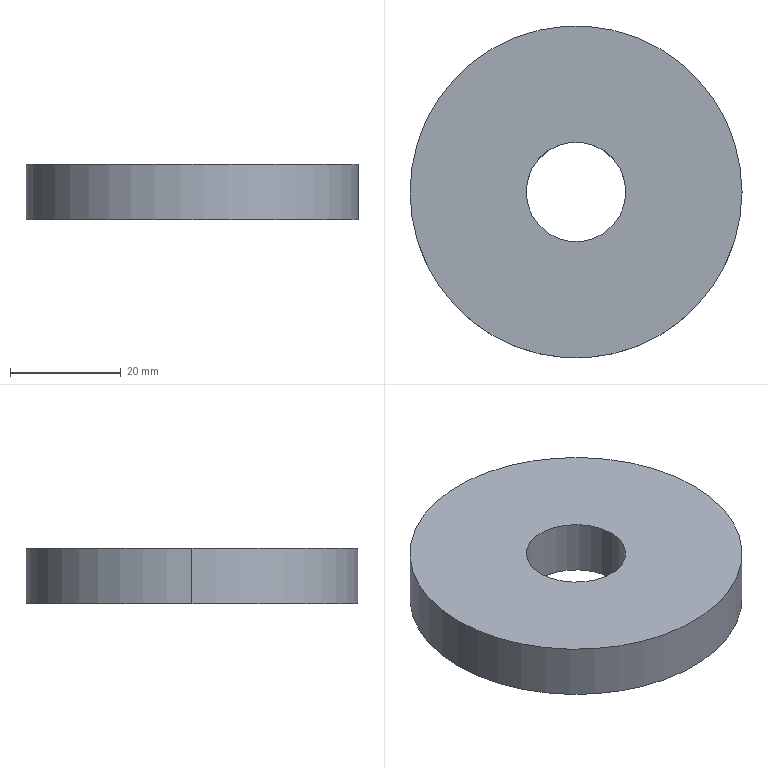Part | STEP file | Pressing pad | 1 solid | 6 faces | box 60 x 60 x 10 mm | volume 25730 mm3 | cylinder 4 | plane 2 | commonest cylinder face diameters 18 x2 60 x2
STEP:
#1=CARTESIAN_POINT('',(0.,0.,0.));
#2=DIRECTION('',(0.,0.,1.));
#3=DIRECTION('',(1.,0.,0.));
#4=AXIS2_PLACEMENT_3D('',#1,#2,#3);
#5=CARTESIAN_POINT('',(-9.,0.,10.));
#6=VERTEX_POINT('',#5);
#7=CARTESIAN_POINT('',(-9.,0.,0.));
#8=VERTEX_POINT('',#7);
#9=CARTESIAN_POINT('',(-9.,0.,10.));
#10=DIRECTION('',(0.,0.,-1.));
#11=VECTOR('',#10,1.);
#12=LINE('',#9,#11);
#13=CARTESIAN_POINT('',(0.,0.,10.));
#14=DIRECTION('',(0.,0.,-1.));
#15=DIRECTION('',(-1.,0.,0.));
#16=AXIS2_PLACEMENT_3D('',#13,#14,#15);
#17=CYLINDRICAL_SURFACE('',#16,9.);
#18=CARTESIAN_POINT('',(6.283,0.));
#19=DIRECTION('',(0.,1.));
#20=VECTOR('',#19,1.);
#21=LINE('',#18,#20);
#22=(GEOMETRIC_REPRESENTATION_CONTEXT(2)PARAMETRIC_REPRESENTATION_CONTEXT()REPRESENTATION_CONTEXT('',''));
#23=DEFINITIONAL_REPRESENTATION('',(#21),#22);
#24=PCURVE('',#17,#23);
#25=CARTESIAN_POINT('',(0.,0.,10.));
#26=DIRECTION('',(0.,0.,-1.));
#27=DIRECTION('',(-1.,0.,0.));
#28=AXIS2_PLACEMENT_3D('',#25,#26,#27);
#29=CYLINDRICAL_SURFACE('',#28,9.);
#30=CARTESIAN_POINT('',(0.,0.));
#31=DIRECTION('',(0.,1.));
#32=VECTOR('',#31,1.);
#33=LINE('',#30,#32);
#34=(GEOMETRIC_REPRESENTATION_CONTEXT(2)PARAMETRIC_REPRESENTATION_CONTEXT()REPRESENTATION_CONTEXT('',''));
#35=DEFINITIONAL_REPRESENTATION('',(#33),#34);
#36=PCURVE('',#29,#35);
#37=SURFACE_CURVE('',#12,(#24,#36),.PCURVE_S1.);
#38=EDGE_CURVE('',#6,#8,#37,.T.);
#39=ORIENTED_EDGE('',*,*,#38,.T.);
#40=CARTESIAN_POINT('',(9.,0.,0.));
#41=VERTEX_POINT('',#40);
#42=CARTESIAN_POINT('',(0.,0.,0.));
#43=DIRECTION('',(0.,0.,1.));
#44=DIRECTION('',(1.,0.,0.));
#45=AXIS2_PLACEMENT_3D('',#42,#43,#44);
#46=CIRCLE('',#45,9.);
#47=CARTESIAN_POINT('',(9.425,10.));
#48=DIRECTION('',(-1.,0.));
#49=VECTOR('',#48,1.);
#50=LINE('',#47,#49);
#51=(GEOMETRIC_REPRESENTATION_CONTEXT(2)PARAMETRIC_REPRESENTATION_CONTEXT()REPRESENTATION_CONTEXT('',''));
#52=DEFINITIONAL_REPRESENTATION('',(#50),#51);
#53=PCURVE('',#17,#52);
#54=CARTESIAN_POINT('',(0.,0.,0.));
#55=DIRECTION('',(0.,0.,1.));
#56=DIRECTION('',(1.,0.,0.));
#57=AXIS2_PLACEMENT_3D('',#54,#55,#56);
#58=PLANE('',#57);
#59=CARTESIAN_POINT('',(0.,0.));
#60=DIRECTION('',(1.,0.));
#61=AXIS2_PLACEMENT_2D('',#59,#60);
#62=CIRCLE('',#61,9.);
#63=(GEOMETRIC_REPRESENTATION_CONTEXT(2)PARAMETRIC_REPRESENTATION_CONTEXT()REPRESENTATION_CONTEXT('',''));
#64=DEFINITIONAL_REPRESENTATION('',(#62),#63);
#65=PCURVE('',#58,#64);
#66=SURFACE_CURVE('',#46,(#53,#65),.PCURVE_S1.);
#67=EDGE_CURVE('',#8,#41,#66,.T.);
#68=ORIENTED_EDGE('',*,*,#67,.T.);
#69=CARTESIAN_POINT('',(9.,0.,10.));
#70=VERTEX_POINT('',#69);
#71=CARTESIAN_POINT('',(9.,0.,10.));
#72=DIRECTION('',(0.,0.,-1.));
#73=VECTOR('',#72,1.);
#74=LINE('',#71,#73);
#75=CARTESIAN_POINT('',(3.142,0.));
#76=DIRECTION('',(0.,1.));
#77=VECTOR('',#76,1.);
#78=LINE('',#75,#77);
#79=(GEOMETRIC_REPRESENTATION_CONTEXT(2)PARAMETRIC_REPRESENTATION_CONTEXT()REPRESENTATION_CONTEXT('',''));
#80=DEFINITIONAL_REPRESENTATION('',(#78),#79);
#81=PCURVE('',#17,#80);
#82=CARTESIAN_POINT('',(3.142,0.));
#83=DIRECTION('',(0.,1.));
#84=VECTOR('',#83,1.);
#85=LINE('',#82,#84);
#86=(GEOMETRIC_REPRESENTATION_CONTEXT(2)PARAMETRIC_REPRESENTATION_CONTEXT()REPRESENTATION_CONTEXT('',''));
#87=DEFINITIONAL_REPRESENTATION('',(#85),#86);
#88=PCURVE('',#29,#87);
#89=SURFACE_CURVE('',#74,(#81,#88),.PCURVE_S1.);
#90=EDGE_CURVE('',#70,#41,#89,.T.);
#91=ORIENTED_EDGE('',*,*,#90,.F.);
#92=CARTESIAN_POINT('',(0.,0.,10.));
#93=DIRECTION('',(0.,0.,1.));
#94=DIRECTION('',(1.,0.,0.));
#95=AXIS2_PLACEMENT_3D('',#92,#93,#94);
#96=CIRCLE('',#95,9.);
#97=CARTESIAN_POINT('',(9.425,0.));
#98=DIRECTION('',(-1.,0.));
#99=VECTOR('',#98,1.);
#100=LINE('',#97,#99);
#101=(GEOMETRIC_REPRESENTATION_CONTEXT(2)PARAMETRIC_REPRESENTATION_CONTEXT()REPRESENTATION_CONTEXT('',''));
#102=DEFINITIONAL_REPRESENTATION('',(#100),#101);
#103=PCURVE('',#17,#102);
#104=CARTESIAN_POINT('',(0.,0.,10.));
#105=DIRECTION('',(0.,0.,1.));
#106=DIRECTION('',(1.,0.,0.));
#107=AXIS2_PLACEMENT_3D('',#104,#105,#106);
#108=PLANE('',#107);
#109=CARTESIAN_POINT('',(0.,0.));
#110=DIRECTION('',(1.,0.));
#111=AXIS2_PLACEMENT_2D('',#109,#110);
#112=CIRCLE('',#111,9.);
#113=(GEOMETRIC_REPRESENTATION_CONTEXT(2)PARAMETRIC_REPRESENTATION_CONTEXT()REPRESENTATION_CONTEXT('',''));
#114=DEFINITIONAL_REPRESENTATION('',(#112),#113);
#115=PCURVE('',#108,#114);
#116=SURFACE_CURVE('',#96,(#103,#115),.PCURVE_S1.);
#117=EDGE_CURVE('',#6,#70,#116,.T.);
#118=ORIENTED_EDGE('',*,*,#117,.F.);
#119=EDGE_LOOP('',(#39,#68,#91,#118));
#120=FACE_BOUND('',#119,.F.);
#121=ADVANCED_FACE('',(#120),#17,.F.);
#122=CARTESIAN_POINT('',(30.,0.,10.));
#123=VERTEX_POINT('',#122);
#124=CARTESIAN_POINT('',(-30.,0.,10.));
#125=VERTEX_POINT('',#124);
#126=CARTESIAN_POINT('',(0.,0.,10.));
#127=DIRECTION('',(0.,0.,1.));
#128=DIRECTION('',(1.,0.,0.));
#129=AXIS2_PLACEMENT_3D('',#126,#127,#128);
#130=CIRCLE('',#129,30.);
#131=CARTESIAN_POINT('',(0.,0.,10.));
#132=DIRECTION('',(0.,0.,-1.));
#133=DIRECTION('',(-1.,0.,0.));
#134=AXIS2_PLACEMENT_3D('',#131,#132,#133);
#135=CYLINDRICAL_SURFACE('',#134,30.);
#136=CARTESIAN_POINT('',(3.142,0.));
#137=DIRECTION('',(-1.,0.));
#138=VECTOR('',#137,1.);
#139=LINE('',#136,#138);
#140=(GEOMETRIC_REPRESENTATION_CONTEXT(2)PARAMETRIC_REPRESENTATION_CONTEXT()REPRESENTATION_CONTEXT('',''));
#141=DEFINITIONAL_REPRESENTATION('',(#139),#140);
#142=PCURVE('',#135,#141);
#143=CARTESIAN_POINT('',(0.,0.));
#144=DIRECTION('',(1.,0.));
#145=AXIS2_PLACEMENT_2D('',#143,#144);
#146=CIRCLE('',#145,30.);
#147=(GEOMETRIC_REPRESENTATION_CONTEXT(2)PARAMETRIC_REPRESENTATION_CONTEXT()REPRESENTATION_CONTEXT('',''));
#148=DEFINITIONAL_REPRESENTATION('',(#146),#147);
#149=PCURVE('',#108,#148);
#150=SURFACE_CURVE('',#130,(#142,#149),.PCURVE_S1.);
#151=EDGE_CURVE('',#123,#125,#150,.T.);
#152=ORIENTED_EDGE('',*,*,#151,.F.);
#153=CARTESIAN_POINT('',(30.,0.,0.));
#154=VERTEX_POINT('',#153);
#155=CARTESIAN_POINT('',(30.,0.,10.));
#156=DIRECTION('',(0.,0.,-1.));
#157=VECTOR('',#156,1.);
#158=LINE('',#155,#157);
#159=CARTESIAN_POINT('',(3.142,0.));
#160=DIRECTION('',(0.,1.));
#161=VECTOR('',#160,1.);
#162=LINE('',#159,#161);
#163=(GEOMETRIC_REPRESENTATION_CONTEXT(2)PARAMETRIC_REPRESENTATION_CONTEXT()REPRESENTATION_CONTEXT('',''));
#164=DEFINITIONAL_REPRESENTATION('',(#162),#163);
#165=PCURVE('',#135,#164);
#166=CARTESIAN_POINT('',(0.,0.,10.));
#167=DIRECTION('',(0.,0.,-1.));
#168=DIRECTION('',(-1.,0.,0.));
#169=AXIS2_PLACEMENT_3D('',#166,#167,#168);
#170=CYLINDRICAL_SURFACE('',#169,30.);
#171=CARTESIAN_POINT('',(3.142,0.));
#172=DIRECTION('',(0.,1.));
#173=VECTOR('',#172,1.);
#174=LINE('',#171,#173);
#175=(GEOMETRIC_REPRESENTATION_CONTEXT(2)PARAMETRIC_REPRESENTATION_CONTEXT()REPRESENTATION_CONTEXT('',''));
#176=DEFINITIONAL_REPRESENTATION('',(#174),#175);
#177=PCURVE('',#170,#176);
#178=SURFACE_CURVE('',#158,(#165,#177),.PCURVE_S1.);
#179=EDGE_CURVE('',#123,#154,#178,.T.);
#180=ORIENTED_EDGE('',*,*,#179,.T.);
#181=CARTESIAN_POINT('',(-30.,0.,0.));
#182=VERTEX_POINT('',#181);
#183=CARTESIAN_POINT('',(0.,0.,0.));
#184=DIRECTION('',(0.,0.,1.));
#185=DIRECTION('',(1.,0.,0.));
#186=AXIS2_PLACEMENT_3D('',#183,#184,#185);
#187=CIRCLE('',#186,30.);
#188=CARTESIAN_POINT('',(3.142,10.));
#189=DIRECTION('',(-1.,0.));
#190=VECTOR('',#189,1.);
#191=LINE('',#188,#190);
#192=(GEOMETRIC_REPRESENTATION_CONTEXT(2)PARAMETRIC_REPRESENTATION_CONTEXT()REPRESENTATION_CONTEXT('',''));
#193=DEFINITIONAL_REPRESENTATION('',(#191),#192);
#194=PCURVE('',#135,#193);
#195=CARTESIAN_POINT('',(0.,0.));
#196=DIRECTION('',(1.,0.));
#197=AXIS2_PLACEMENT_2D('',#195,#196);
#198=CIRCLE('',#197,30.);
#199=(GEOMETRIC_REPRESENTATION_CONTEXT(2)PARAMETRIC_REPRESENTATION_CONTEXT()REPRESENTATION_CONTEXT('',''));
#200=DEFINITIONAL_REPRESENTATION('',(#198),#199);
#201=PCURVE('',#58,#200);
#202=SURFACE_CURVE('',#187,(#194,#201),.PCURVE_S1.);
#203=EDGE_CURVE('',#154,#182,#202,.T.);
#204=ORIENTED_EDGE('',*,*,#203,.T.);
#205=CARTESIAN_POINT('',(-30.,0.,10.));
#206=DIRECTION('',(0.,0.,-1.));
#207=VECTOR('',#206,1.);
#208=LINE('',#205,#207);
#209=CARTESIAN_POINT('',(0.,0.));
#210=DIRECTION('',(0.,1.));
#211=VECTOR('',#210,1.);
#212=LINE('',#209,#211);
#213=(GEOMETRIC_REPRESENTATION_CONTEXT(2)PARAMETRIC_REPRESENTATION_CONTEXT()REPRESENTATION_CONTEXT('',''));
#214=DEFINITIONAL_REPRESENTATION('',(#212),#213);
#215=PCURVE('',#135,#214);
#216=CARTESIAN_POINT('',(6.283,0.));
#217=DIRECTION('',(0.,1.));
#218=VECTOR('',#217,1.);
#219=LINE('',#216,#218);
#220=(GEOMETRIC_REPRESENTATION_CONTEXT(2)PARAMETRIC_REPRESENTATION_CONTEXT()REPRESENTATION_CONTEXT('',''));
#221=DEFINITIONAL_REPRESENTATION('',(#219),#220);
#222=PCURVE('',#170,#221);
#223=SURFACE_CURVE('',#208,(#215,#222),.PCURVE_S1.);
#224=EDGE_CURVE('',#125,#182,#223,.T.);
#225=ORIENTED_EDGE('',*,*,#224,.F.);
#226=EDGE_LOOP('',(#152,#180,#204,#225));
#227=FACE_BOUND('',#226,.T.);
#228=ADVANCED_FACE('',(#227),#135,.T.);
#229=CARTESIAN_POINT('',(0.,0.,10.));
#230=DIRECTION('',(0.,0.,1.));
#231=DIRECTION('',(1.,0.,0.));
#232=AXIS2_PLACEMENT_3D('',#229,#230,#231);
#233=CIRCLE('',#232,30.);
#234=CARTESIAN_POINT('',(0.,0.));
#235=DIRECTION('',(1.,0.));
#236=AXIS2_PLACEMENT_2D('',#234,#235);
#237=CIRCLE('',#236,30.);
#238=(GEOMETRIC_REPRESENTATION_CONTEXT(2)PARAMETRIC_REPRESENTATION_CONTEXT()REPRESENTATION_CONTEXT('',''));
#239=DEFINITIONAL_REPRESENTATION('',(#237),#238);
#240=PCURVE('',#108,#239);
#241=CARTESIAN_POINT('',(9.425,0.));
#242=DIRECTION('',(-1.,0.));
#243=VECTOR('',#242,1.);
#244=LINE('',#241,#243);
#245=(GEOMETRIC_REPRESENTATION_CONTEXT(2)PARAMETRIC_REPRESENTATION_CONTEXT()REPRESENTATION_CONTEXT('',''));
#246=DEFINITIONAL_REPRESENTATION('',(#244),#245);
#247=PCURVE('',#170,#246);
#248=SURFACE_CURVE('',#233,(#240,#247),.PCURVE_S1.);
#249=EDGE_CURVE('',#125,#123,#248,.T.);
#250=ORIENTED_EDGE('',*,*,#249,.T.);
#251=ORIENTED_EDGE('',*,*,#151,.T.);
#252=EDGE_LOOP('',(#250,#251));
#253=FACE_BOUND('',#252,.T.);
#254=ORIENTED_EDGE('',*,*,#117,.F.);
#255=CARTESIAN_POINT('',(0.,0.,10.));
#256=DIRECTION('',(0.,0.,1.));
#257=DIRECTION('',(1.,0.,0.));
#258=AXIS2_PLACEMENT_3D('',#255,#256,#257);
#259=CIRCLE('',#258,9.);
#260=CARTESIAN_POINT('',(0.,0.));
#261=DIRECTION('',(1.,0.));
#262=AXIS2_PLACEMENT_2D('',#260,#261);
#263=CIRCLE('',#262,9.);
#264=(GEOMETRIC_REPRESENTATION_CONTEXT(2)PARAMETRIC_REPRESENTATION_CONTEXT()REPRESENTATION_CONTEXT('',''));
#265=DEFINITIONAL_REPRESENTATION('',(#263),#264);
#266=PCURVE('',#108,#265);
#267=CARTESIAN_POINT('',(3.142,0.));
#268=DIRECTION('',(-1.,0.));
#269=VECTOR('',#268,1.);
#270=LINE('',#267,#269);
#271=(GEOMETRIC_REPRESENTATION_CONTEXT(2)PARAMETRIC_REPRESENTATION_CONTEXT()REPRESENTATION_CONTEXT('',''));
#272=DEFINITIONAL_REPRESENTATION('',(#270),#271);
#273=PCURVE('',#29,#272);
#274=SURFACE_CURVE('',#259,(#266,#273),.PCURVE_S1.);
#275=EDGE_CURVE('',#70,#6,#274,.T.);
#276=ORIENTED_EDGE('',*,*,#275,.F.);
#277=EDGE_LOOP('',(#254,#276));
#278=FACE_BOUND('',#277,.T.);
#279=ADVANCED_FACE('',(#253,#278),#108,.T.);
#280=CARTESIAN_POINT('',(0.,0.,0.));
#281=DIRECTION('',(0.,0.,1.));
#282=DIRECTION('',(1.,0.,0.));
#283=AXIS2_PLACEMENT_3D('',#280,#281,#282);
#284=CIRCLE('',#283,30.);
#285=CARTESIAN_POINT('',(0.,0.));
#286=DIRECTION('',(1.,0.));
#287=AXIS2_PLACEMENT_2D('',#285,#286);
#288=CIRCLE('',#287,30.);
#289=(GEOMETRIC_REPRESENTATION_CONTEXT(2)PARAMETRIC_REPRESENTATION_CONTEXT()REPRESENTATION_CONTEXT('',''));
#290=DEFINITIONAL_REPRESENTATION('',(#288),#289);
#291=PCURVE('',#58,#290);
#292=CARTESIAN_POINT('',(9.425,10.));
#293=DIRECTION('',(-1.,0.));
#294=VECTOR('',#293,1.);
#295=LINE('',#292,#294);
#296=(GEOMETRIC_REPRESENTATION_CONTEXT(2)PARAMETRIC_REPRESENTATION_CONTEXT()REPRESENTATION_CONTEXT('',''));
#297=DEFINITIONAL_REPRESENTATION('',(#295),#296);
#298=PCURVE('',#170,#297);
#299=SURFACE_CURVE('',#284,(#291,#298),.PCURVE_S1.);
#300=EDGE_CURVE('',#182,#154,#299,.T.);
#301=ORIENTED_EDGE('',*,*,#300,.F.);
#302=ORIENTED_EDGE('',*,*,#203,.F.);
#303=EDGE_LOOP('',(#301,#302));
#304=FACE_BOUND('',#303,.T.);
#305=ORIENTED_EDGE('',*,*,#67,.T.);
#306=CARTESIAN_POINT('',(0.,0.,0.));
#307=DIRECTION('',(0.,0.,1.));
#308=DIRECTION('',(1.,0.,0.));
#309=AXIS2_PLACEMENT_3D('',#306,#307,#308);
#310=CIRCLE('',#309,9.);
#311=CARTESIAN_POINT('',(0.,0.));
#312=DIRECTION('',(1.,0.));
#313=AXIS2_PLACEMENT_2D('',#311,#312);
#314=CIRCLE('',#313,9.);
#315=(GEOMETRIC_REPRESENTATION_CONTEXT(2)PARAMETRIC_REPRESENTATION_CONTEXT()REPRESENTATION_CONTEXT('',''));
#316=DEFINITIONAL_REPRESENTATION('',(#314),#315);
#317=PCURVE('',#58,#316);
#318=CARTESIAN_POINT('',(3.142,10.));
#319=DIRECTION('',(-1.,0.));
#320=VECTOR('',#319,1.);
#321=LINE('',#318,#320);
#322=(GEOMETRIC_REPRESENTATION_CONTEXT(2)PARAMETRIC_REPRESENTATION_CONTEXT()REPRESENTATION_CONTEXT('',''));
#323=DEFINITIONAL_REPRESENTATION('',(#321),#322);
#324=PCURVE('',#29,#323);
#325=SURFACE_CURVE('',#310,(#317,#324),.PCURVE_S1.);
#326=EDGE_CURVE('',#41,#8,#325,.T.);
#327=ORIENTED_EDGE('',*,*,#326,.T.);
#328=EDGE_LOOP('',(#305,#327));
#329=FACE_BOUND('',#328,.T.);
#330=ADVANCED_FACE('',(#304,#329),#58,.F.);
#331=ORIENTED_EDGE('',*,*,#179,.F.);
#332=ORIENTED_EDGE('',*,*,#249,.F.);
#333=ORIENTED_EDGE('',*,*,#224,.T.);
#334=ORIENTED_EDGE('',*,*,#300,.T.);
#335=EDGE_LOOP('',(#331,#332,#333,#334));
#336=FACE_BOUND('',#335,.T.);
#337=ADVANCED_FACE('',(#336),#170,.T.);
#338=ORIENTED_EDGE('',*,*,#326,.T.);
#339=ORIENTED_EDGE('',*,*,#38,.F.);
#340=ORIENTED_EDGE('',*,*,#275,.F.);
#341=ORIENTED_EDGE('',*,*,#90,.T.);
#342=EDGE_LOOP('',(#338,#339,#340,#341));
#343=FACE_BOUND('',#342,.F.);
#344=ADVANCED_FACE('',(#343),#29,.F.);
#345=CLOSED_SHELL('',(#121,#228,#279,#330,#337,#344));
#346=MANIFOLD_SOLID_BREP('',#345);
#347=(LENGTH_UNIT()NAMED_UNIT(*)SI_UNIT(.MILLI.,.METRE.));
#348=UNCERTAINTY_MEASURE_WITH_UNIT(LENGTH_MEASURE(0.0000001),#347,'','');
#349=(NAMED_UNIT(*)PLANE_ANGLE_UNIT()SI_UNIT($,.RADIAN.));
#350=(NAMED_UNIT(*)SI_UNIT($,.STERADIAN.)SOLID_ANGLE_UNIT());
#351=(GEOMETRIC_REPRESENTATION_CONTEXT(3)GLOBAL_UNCERTAINTY_ASSIGNED_CONTEXT((#348))GLOBAL_UNIT_ASSIGNED_CONTEXT((#347,#349,#350))REPRESENTATION_CONTEXT('',''));
#352=ADVANCED_BREP_SHAPE_REPRESENTATION('',(#4,#346),#351);